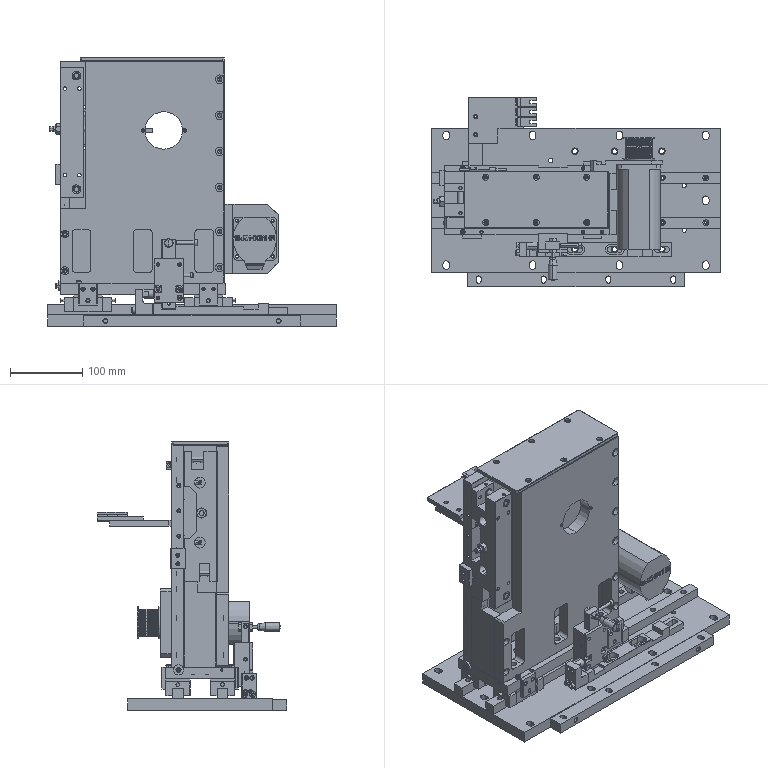Part | NX | 74 solids | 4373 faces | volume 5118131 mm3 | plane 2214 | cylinder 1473 | cone 632 | spline 44 | sphere 6 | torus 4 | commonest cylinder face diameters 5 x427 3.3 x150 4.5 x64 6.6 x54 0.5 x52 6.55 x52